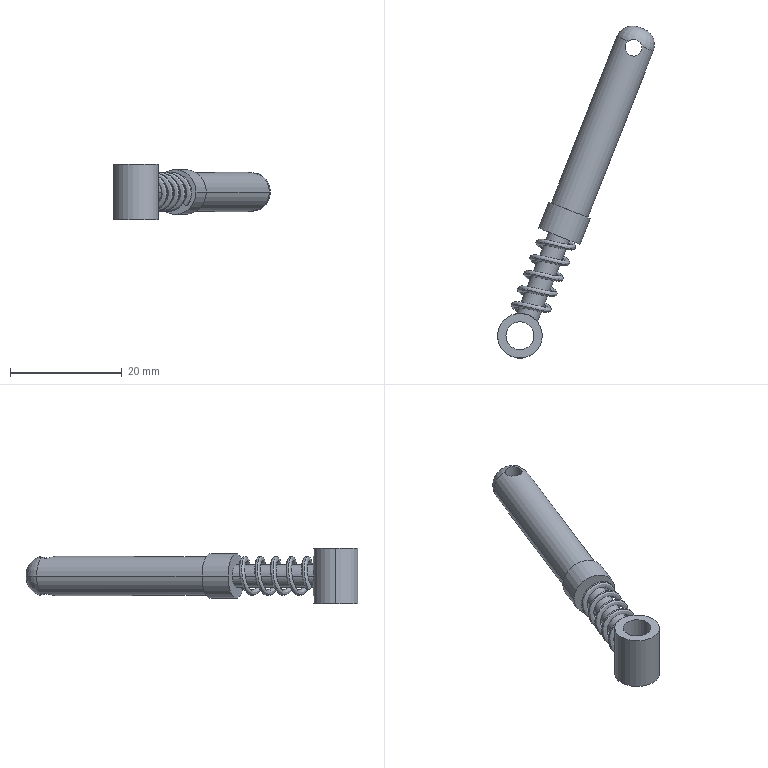Part | SolidWorks | features ICE 4, 3DProfileFeature 1, Extrusion 1, Fillet 1, Helix 1, Sweep 1 | 2 solids | 23 faces | box 28.061 x 59.393 x 10 mm | volume 2085 mm3 | cylinder 12 | plane 7 | torus 2 | spline 2 | commonest cylinder face diameters 8 x4 3 x2 4 x2 5 x2 7 x2